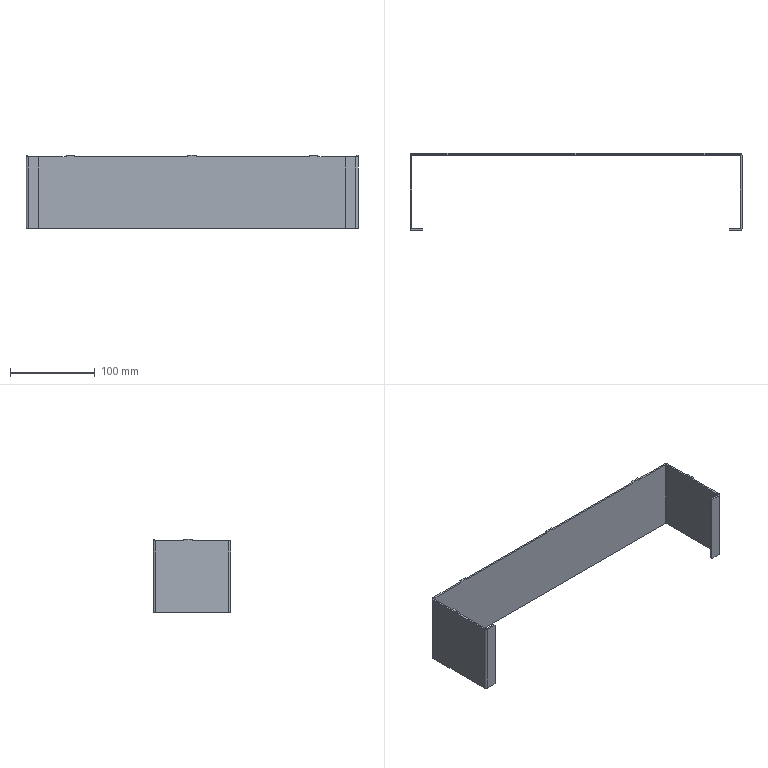Part | STEP file | xzz-002 | 1 solid | 42 faces | box 392 x 91.5 x 87 mm | volume 101252 mm3 | plane 34 | cylinder 8 | commonest cylinder face diameters 1 x4 5 x4
STEP:
#1=CARTESIAN_POINT('',(216.5,24.,85.));
#2=VERTEX_POINT('',#1);
#3=CARTESIAN_POINT('',(216.5,24.,0.));
#4=VERTEX_POINT('',#3);
#5=CARTESIAN_POINT('',(216.5,24.,85.));
#6=DIRECTION('',(0.,0.,-1.));
#7=VECTOR('',#6,1000.);
#8=LINE('',#5,#7);
#9=EDGE_CURVE('',#2,#4,#8,.T.);
#10=ORIENTED_EDGE('',*,*,#9,.F.);
#11=CARTESIAN_POINT('',(171.7,24.,85.));
#12=VERTEX_POINT('',#11);
#13=CARTESIAN_POINT('',(-173.,24.,85.));
#14=DIRECTION('',(1.,0.,0.));
#15=VECTOR('',#14,1000.);
#16=LINE('',#13,#15);
#17=EDGE_CURVE('',#12,#2,#16,.T.);
#18=ORIENTED_EDGE('',*,*,#17,.F.);
#19=CARTESIAN_POINT('',(171.7,24.,87.));
#20=VERTEX_POINT('',#19);
#21=CARTESIAN_POINT('',(171.7,24.,85.));
#22=DIRECTION('',(0.,0.,-1.));
#23=VECTOR('',#22,1000.);
#24=LINE('',#21,#23);
#25=EDGE_CURVE('',#20,#12,#24,.T.);
#26=ORIENTED_EDGE('',*,*,#25,.F.);
#27=CARTESIAN_POINT('',(161.7,24.,87.));
#28=VERTEX_POINT('',#27);
#29=CARTESIAN_POINT('',(-173.,24.,87.));
#30=DIRECTION('',(1.,0.,0.));
#31=VECTOR('',#30,1000.);
#32=LINE('',#29,#31);
#33=EDGE_CURVE('',#28,#20,#32,.T.);
#34=ORIENTED_EDGE('',*,*,#33,.F.);
#35=CARTESIAN_POINT('',(161.7,24.,85.));
#36=VERTEX_POINT('',#35);
#37=CARTESIAN_POINT('',(161.7,24.,85.));
#38=DIRECTION('',(0.,0.,1.));
#39=VECTOR('',#38,1000.);
#40=LINE('',#37,#39);
#41=EDGE_CURVE('',#36,#28,#40,.T.);
#42=ORIENTED_EDGE('',*,*,#41,.F.);
#43=CARTESIAN_POINT('',(28.,24.,85.));
#44=VERTEX_POINT('',#43);
#45=CARTESIAN_POINT('',(-173.,24.,85.));
#46=DIRECTION('',(1.,0.,0.));
#47=VECTOR('',#46,1000.);
#48=LINE('',#45,#47);
#49=EDGE_CURVE('',#44,#36,#48,.T.);
#50=ORIENTED_EDGE('',*,*,#49,.F.);
#51=CARTESIAN_POINT('',(28.,24.,87.));
#52=VERTEX_POINT('',#51);
#53=CARTESIAN_POINT('',(28.,24.,85.));
#54=DIRECTION('',(0.,0.,-1.));
#55=VECTOR('',#54,1000.);
#56=LINE('',#53,#55);
#57=EDGE_CURVE('',#52,#44,#56,.T.);
#58=ORIENTED_EDGE('',*,*,#57,.F.);
#59=CARTESIAN_POINT('',(18.,24.,87.));
#60=VERTEX_POINT('',#59);
#61=CARTESIAN_POINT('',(-173.,24.,87.));
#62=DIRECTION('',(1.,0.,0.));
#63=VECTOR('',#62,1000.);
#64=LINE('',#61,#63);
#65=EDGE_CURVE('',#60,#52,#64,.T.);
#66=ORIENTED_EDGE('',*,*,#65,.F.);
#67=CARTESIAN_POINT('',(18.,24.,85.));
#68=VERTEX_POINT('',#67);
#69=CARTESIAN_POINT('',(18.,24.,85.));
#70=DIRECTION('',(0.,0.,1.));
#71=VECTOR('',#70,1000.);
#72=LINE('',#69,#71);
#73=EDGE_CURVE('',#68,#60,#72,.T.);
#74=ORIENTED_EDGE('',*,*,#73,.F.);
#75=CARTESIAN_POINT('',(-115.7,24.,85.));
#76=VERTEX_POINT('',#75);
#77=CARTESIAN_POINT('',(-173.,24.,85.));
#78=DIRECTION('',(1.,0.,0.));
#79=VECTOR('',#78,1000.);
#80=LINE('',#77,#79);
#81=EDGE_CURVE('',#76,#68,#80,.T.);
#82=ORIENTED_EDGE('',*,*,#81,.F.);
#83=CARTESIAN_POINT('',(-115.7,24.,87.));
#84=VERTEX_POINT('',#83);
#85=CARTESIAN_POINT('',(-115.7,24.,85.));
#86=DIRECTION('',(0.,0.,-1.));
#87=VECTOR('',#86,1000.);
#88=LINE('',#85,#87);
#89=EDGE_CURVE('',#84,#76,#88,.T.);
#90=ORIENTED_EDGE('',*,*,#89,.F.);
#91=CARTESIAN_POINT('',(-125.7,24.,87.));
#92=VERTEX_POINT('',#91);
#93=CARTESIAN_POINT('',(-173.,24.,87.));
#94=DIRECTION('',(1.,0.,0.));
#95=VECTOR('',#94,1000.);
#96=LINE('',#93,#95);
#97=EDGE_CURVE('',#92,#84,#96,.T.);
#98=ORIENTED_EDGE('',*,*,#97,.F.);
#99=CARTESIAN_POINT('',(-125.7,24.,85.));
#100=VERTEX_POINT('',#99);
#101=CARTESIAN_POINT('',(-125.7,24.,85.));
#102=DIRECTION('',(0.,0.,1.));
#103=VECTOR('',#102,1000.);
#104=LINE('',#101,#103);
#105=EDGE_CURVE('',#100,#92,#104,.T.);
#106=ORIENTED_EDGE('',*,*,#105,.F.);
#107=CARTESIAN_POINT('',(-170.5,24.,85.));
#108=VERTEX_POINT('',#107);
#109=CARTESIAN_POINT('',(-173.,24.,85.));
#110=DIRECTION('',(1.,0.,0.));
#111=VECTOR('',#110,1000.);
#112=LINE('',#109,#111);
#113=EDGE_CURVE('',#108,#100,#112,.T.);
#114=ORIENTED_EDGE('',*,*,#113,.F.);
#115=CARTESIAN_POINT('',(-170.5,24.,0.));
#116=VERTEX_POINT('',#115);
#117=CARTESIAN_POINT('',(-170.5,24.,85.));
#118=DIRECTION('',(0.,0.,1.));
#119=VECTOR('',#118,1000.);
#120=LINE('',#117,#119);
#121=EDGE_CURVE('',#116,#108,#120,.T.);
#122=ORIENTED_EDGE('',*,*,#121,.F.);
#123=CARTESIAN_POINT('',(-173.,24.,0.));
#124=DIRECTION('',(-1.,0.,0.));
#125=VECTOR('',#124,1000.);
#126=LINE('',#123,#125);
#127=EDGE_CURVE('',#4,#116,#126,.T.);
#128=ORIENTED_EDGE('',*,*,#127,.F.);
#129=EDGE_LOOP('',(#10,#18,#26,#34,#42,#50,#58,#66,#74,#82,#90,#98,#106,#114,#122,#128));
#130=FACE_OUTER_BOUND('',#129,.T.);
#131=CARTESIAN_POINT('',(-173.,24.,85.));
#132=DIRECTION('',(0.,1.,0.));
#133=DIRECTION('',(0.,0.,1.));
#134=AXIS2_PLACEMENT_3D('',#131,#132,#133);
#135=PLANE('',#134);
#136=ADVANCED_FACE('',(#130),#135,.F.);
#137=ORIENTED_EDGE('',*,*,#127,.T.);
#138=CARTESIAN_POINT('',(-171.,23.5,0.));
#139=VERTEX_POINT('',#138);
#140=CARTESIAN_POINT('',(-170.5,23.5,0.));
#141=DIRECTION('',(0.,0.,1.));
#142=DIRECTION('',(-1.,0.,0.));
#143=AXIS2_PLACEMENT_3D('',#140,#141,#142);
#144=CIRCLE('',#143,0.5);
#145=EDGE_CURVE('',#116,#139,#144,.T.);
#146=ORIENTED_EDGE('',*,*,#145,.T.);
#147=CARTESIAN_POINT('',(-171.,-63.,0.));
#148=VERTEX_POINT('',#147);
#149=CARTESIAN_POINT('',(-171.,26.,0.));
#150=DIRECTION('',(0.,-1.,0.));
#151=VECTOR('',#150,1000.);
#152=LINE('',#149,#151);
#153=EDGE_CURVE('',#139,#148,#152,.T.);
#154=ORIENTED_EDGE('',*,*,#153,.T.);
#155=CARTESIAN_POINT('',(-170.5,-63.5,0.));
#156=VERTEX_POINT('',#155);
#157=CARTESIAN_POINT('',(-170.5,-63.,0.));
#158=DIRECTION('',(0.,0.,1.));
#159=DIRECTION('',(-1.,0.,0.));
#160=AXIS2_PLACEMENT_3D('',#157,#158,#159);
#161=CIRCLE('',#160,0.5);
#162=EDGE_CURVE('',#148,#156,#161,.T.);
#163=ORIENTED_EDGE('',*,*,#162,.T.);
#164=CARTESIAN_POINT('',(-158.,-63.5,0.));
#165=VERTEX_POINT('',#164);
#166=CARTESIAN_POINT('',(-173.,-63.5,0.));
#167=DIRECTION('',(1.,0.,0.));
#168=VECTOR('',#167,1000.);
#169=LINE('',#166,#168);
#170=EDGE_CURVE('',#156,#165,#169,.T.);
#171=ORIENTED_EDGE('',*,*,#170,.T.);
#172=CARTESIAN_POINT('',(-158.,-65.5,0.));
#173=VERTEX_POINT('',#172);
#174=CARTESIAN_POINT('',(-158.,-63.,0.));
#175=DIRECTION('',(0.,-1.,0.));
#176=VECTOR('',#175,1000.);
#177=LINE('',#174,#176);
#178=EDGE_CURVE('',#165,#173,#177,.T.);
#179=ORIENTED_EDGE('',*,*,#178,.T.);
#180=CARTESIAN_POINT('',(-170.5,-65.5,0.));
#181=VERTEX_POINT('',#180);
#182=CARTESIAN_POINT('',(-171.,-65.5,0.));
#183=DIRECTION('',(-1.,0.,0.));
#184=VECTOR('',#183,1000.);
#185=LINE('',#182,#184);
#186=EDGE_CURVE('',#173,#181,#185,.T.);
#187=ORIENTED_EDGE('',*,*,#186,.T.);
#188=CARTESIAN_POINT('',(-173.,-63.,0.));
#189=VERTEX_POINT('',#188);
#190=CARTESIAN_POINT('',(-170.5,-63.,0.));
#191=DIRECTION('',(0.,0.,-1.));
#192=DIRECTION('',(-1.,0.,0.));
#193=AXIS2_PLACEMENT_3D('',#190,#191,#192);
#194=CIRCLE('',#193,2.5);
#195=EDGE_CURVE('',#181,#189,#194,.T.);
#196=ORIENTED_EDGE('',*,*,#195,.T.);
#197=CARTESIAN_POINT('',(-173.,23.5,0.));
#198=VERTEX_POINT('',#197);
#199=CARTESIAN_POINT('',(-173.,24.,0.));
#200=DIRECTION('',(0.,1.,0.));
#201=VECTOR('',#200,1000.);
#202=LINE('',#199,#201);
#203=EDGE_CURVE('',#189,#198,#202,.T.);
#204=ORIENTED_EDGE('',*,*,#203,.T.);
#205=CARTESIAN_POINT('',(-170.5,26.,0.));
#206=VERTEX_POINT('',#205);
#207=CARTESIAN_POINT('',(-170.5,23.5,0.));
#208=DIRECTION('',(0.,0.,-1.));
#209=DIRECTION('',(-1.,0.,0.));
#210=AXIS2_PLACEMENT_3D('',#207,#208,#209);
#211=CIRCLE('',#210,2.5);
#212=EDGE_CURVE('',#198,#206,#211,.T.);
#213=ORIENTED_EDGE('',*,*,#212,.T.);
#214=CARTESIAN_POINT('',(216.5,26.,0.));
#215=VERTEX_POINT('',#214);
#216=CARTESIAN_POINT('',(217.,26.,0.));
#217=DIRECTION('',(1.,0.,0.));
#218=VECTOR('',#217,1000.);
#219=LINE('',#216,#218);
#220=EDGE_CURVE('',#206,#215,#219,.T.);
#221=ORIENTED_EDGE('',*,*,#220,.T.);
#222=CARTESIAN_POINT('',(219.,23.5,0.));
#223=VERTEX_POINT('',#222);
#224=CARTESIAN_POINT('',(216.5,23.5,0.));
#225=DIRECTION('',(0.,0.,-1.));
#226=DIRECTION('',(-1.,0.,0.));
#227=AXIS2_PLACEMENT_3D('',#224,#225,#226);
#228=CIRCLE('',#227,2.5);
#229=EDGE_CURVE('',#215,#223,#228,.T.);
#230=ORIENTED_EDGE('',*,*,#229,.T.);
#231=CARTESIAN_POINT('',(219.,-63.,0.));
#232=VERTEX_POINT('',#231);
#233=CARTESIAN_POINT('',(219.,-63.5,0.));
#234=DIRECTION('',(0.,-1.,0.));
#235=VECTOR('',#234,1000.);
#236=LINE('',#233,#235);
#237=EDGE_CURVE('',#223,#232,#236,.T.);
#238=ORIENTED_EDGE('',*,*,#237,.T.);
#239=CARTESIAN_POINT('',(216.5,-65.5,0.));
#240=VERTEX_POINT('',#239);
#241=CARTESIAN_POINT('',(216.5,-63.,0.));
#242=DIRECTION('',(0.,0.,-1.));
#243=DIRECTION('',(-1.,0.,0.));
#244=AXIS2_PLACEMENT_3D('',#241,#242,#243);
#245=CIRCLE('',#244,2.5);
#246=EDGE_CURVE('',#232,#240,#245,.T.);
#247=ORIENTED_EDGE('',*,*,#246,.T.);
#248=CARTESIAN_POINT('',(204.,-65.5,0.));
#249=VERTEX_POINT('',#248);
#250=CARTESIAN_POINT('',(216.5,-65.5,0.));
#251=DIRECTION('',(1.,0.,0.));
#252=VECTOR('',#251,1000.);
#253=LINE('',#250,#252);
#254=EDGE_CURVE('',#249,#240,#253,.T.);
#255=ORIENTED_EDGE('',*,*,#254,.F.);
#256=CARTESIAN_POINT('',(204.,-63.5,0.));
#257=VERTEX_POINT('',#256);
#258=CARTESIAN_POINT('',(204.,-63.,0.));
#259=DIRECTION('',(0.,-1.,0.));
#260=VECTOR('',#259,1000.);
#261=LINE('',#258,#260);
#262=EDGE_CURVE('',#257,#249,#261,.T.);
#263=ORIENTED_EDGE('',*,*,#262,.F.);
#264=CARTESIAN_POINT('',(216.5,-63.5,0.));
#265=VERTEX_POINT('',#264);
#266=CARTESIAN_POINT('',(219.,-63.5,0.));
#267=DIRECTION('',(1.,0.,0.));
#268=VECTOR('',#267,1000.);
#269=LINE('',#266,#268);
#270=EDGE_CURVE('',#257,#265,#269,.T.);
#271=ORIENTED_EDGE('',*,*,#270,.T.);
#272=CARTESIAN_POINT('',(217.,-63.,0.));
#273=VERTEX_POINT('',#272);
#274=CARTESIAN_POINT('',(216.5,-63.,0.));
#275=DIRECTION('',(0.,0.,1.));
#276=DIRECTION('',(-1.,0.,0.));
#277=AXIS2_PLACEMENT_3D('',#274,#275,#276);
#278=CIRCLE('',#277,0.5);
#279=EDGE_CURVE('',#265,#273,#278,.T.);
#280=ORIENTED_EDGE('',*,*,#279,.T.);
#281=CARTESIAN_POINT('',(217.,23.5,0.));
#282=VERTEX_POINT('',#281);
#283=CARTESIAN_POINT('',(217.,26.,0.));
#284=DIRECTION('',(0.,1.,0.));
#285=VECTOR('',#284,1000.);
#286=LINE('',#283,#285);
#287=EDGE_CURVE('',#273,#282,#286,.T.);
#288=ORIENTED_EDGE('',*,*,#287,.T.);
#289=CARTESIAN_POINT('',(216.5,23.5,0.));
#290=DIRECTION('',(0.,0.,1.));
#291=DIRECTION('',(-1.,0.,0.));
#292=AXIS2_PLACEMENT_3D('',#289,#290,#291);
#293=CIRCLE('',#292,0.5);
#294=EDGE_CURVE('',#282,#4,#293,.T.);
#295=ORIENTED_EDGE('',*,*,#294,.T.);
#296=EDGE_LOOP('',(#137,#146,#154,#163,#171,#179,#187,#196,#204,#213,#221,#230,#238,#247,#255,#263,#271,#280,#288,#295));
#297=FACE_OUTER_BOUND('',#296,.T.);
#298=CARTESIAN_POINT('',(217.,23.5,0.));
#299=DIRECTION('',(0.,0.,-1.));
#300=DIRECTION('',(-1.,0.,0.));
#301=AXIS2_PLACEMENT_3D('',#298,#299,#300);
#302=PLANE('',#301);
#303=ADVANCED_FACE('',(#297),#302,.T.);
#304=CARTESIAN_POINT('',(217.,23.5,85.));
#305=VERTEX_POINT('',#304);
#306=CARTESIAN_POINT('',(217.,23.5,85.));
#307=DIRECTION('',(0.,0.,-1.));
#308=VECTOR('',#307,1000.);
#309=LINE('',#306,#308);
#310=EDGE_CURVE('',#305,#282,#309,.T.);
#311=ORIENTED_EDGE('',*,*,#310,.F.);
#312=CARTESIAN_POINT('',(216.5,23.5,85.));
#313=DIRECTION('',(0.,0.,-1.));
#314=DIRECTION('',(-1.,0.,0.));
#315=AXIS2_PLACEMENT_3D('',#312,#313,#314);
#316=CIRCLE('',#315,0.5);
#317=EDGE_CURVE('',#2,#305,#316,.T.);
#318=ORIENTED_EDGE('',*,*,#317,.F.);
#319=ORIENTED_EDGE('',*,*,#9,.T.);
#320=ORIENTED_EDGE('',*,*,#294,.F.);
#321=EDGE_LOOP('',(#311,#318,#319,#320));
#322=FACE_OUTER_BOUND('',#321,.T.);
#323=CARTESIAN_POINT('',(216.5,23.5,85.));
#324=DIRECTION('',(0.,0.,-1.));
#325=DIRECTION('',(-1.,0.,0.));
#326=AXIS2_PLACEMENT_3D('',#323,#324,#325);
#327=CYLINDRICAL_SURFACE('',#326,0.5);
#328=ADVANCED_FACE('',(#322),#327,.F.);
#329=ORIENTED_EDGE('',*,*,#17,.T.);
#330=ORIENTED_EDGE('',*,*,#317,.T.);
#331=CARTESIAN_POINT('',(217.,-10.,85.));
#332=VERTEX_POINT('',#331);
#333=CARTESIAN_POINT('',(217.,26.,85.));
#334=DIRECTION('',(0.,-1.,0.));
#335=VECTOR('',#334,1000.);
#336=LINE('',#333,#335);
#337=EDGE_CURVE('',#305,#332,#336,.T.);
#338=ORIENTED_EDGE('',*,*,#337,.T.);
#339=CARTESIAN_POINT('',(219.,-10.,85.));
#340=VERTEX_POINT('',#339);
#341=CARTESIAN_POINT('',(217.,-10.,85.));
#342=DIRECTION('',(1.,0.,0.));
#343=VECTOR('',#342,1000.);
#344=LINE('',#341,#343);
#345=EDGE_CURVE('',#332,#340,#344,.T.);
#346=ORIENTED_EDGE('',*,*,#345,.T.);
#347=CARTESIAN_POINT('',(219.,23.5,85.));
#348=VERTEX_POINT('',#347);
#349=CARTESIAN_POINT('',(219.,24.,85.));
#350=DIRECTION('',(0.,1.,0.));
#351=VECTOR('',#350,1000.);
#352=LINE('',#349,#351);
#353=EDGE_CURVE('',#340,#348,#352,.T.);
#354=ORIENTED_EDGE('',*,*,#353,.T.);
#355=CARTESIAN_POINT('',(216.5,26.,85.));
#356=VERTEX_POINT('',#355);
#357=CARTESIAN_POINT('',(216.5,23.5,85.));
#358=DIRECTION('',(0.,0.,1.));
#359=DIRECTION('',(-1.,0.,0.));
#360=AXIS2_PLACEMENT_3D('',#357,#358,#359);
#361=CIRCLE('',#360,2.5);
#362=EDGE_CURVE('',#348,#356,#361,.T.);
#363=ORIENTED_EDGE('',*,*,#362,.T.);
#364=CARTESIAN_POINT('',(171.7,26.,85.));
#365=VERTEX_POINT('',#364);
#366=CARTESIAN_POINT('',(-171.,26.,85.));
#367=DIRECTION('',(-1.,0.,0.));
#368=VECTOR('',#367,1000.);
#369=LINE('',#366,#368);
#370=EDGE_CURVE('',#356,#365,#369,.T.);
#371=ORIENTED_EDGE('',*,*,#370,.T.);
#372=CARTESIAN_POINT('',(171.7,23.5,85.));
#373=DIRECTION('',(0.,-1.,0.));
#374=VECTOR('',#373,1000.);
#375=LINE('',#372,#374);
#376=EDGE_CURVE('',#365,#12,#375,.T.);
#377=ORIENTED_EDGE('',*,*,#376,.T.);
#378=EDGE_LOOP('',(#329,#330,#338,#346,#354,#363,#371,#377));
#379=FACE_OUTER_BOUND('',#378,.T.);
#380=CARTESIAN_POINT('',(-171.,23.5,85.));
#381=DIRECTION('',(0.,0.,1.));
#382=DIRECTION('',(1.,0.,0.));
#383=AXIS2_PLACEMENT_3D('',#380,#381,#382);
#384=PLANE('',#383);
#385=ADVANCED_FACE('',(#379),#384,.T.);
#386=CARTESIAN_POINT('',(171.7,26.,87.));
#387=VERTEX_POINT('',#386);
#388=CARTESIAN_POINT('',(171.7,26.,87.));
#389=DIRECTION('',(0.,0.,-1.));
#390=VECTOR('',#389,1000.);
#391=LINE('',#388,#390);
#392=EDGE_CURVE('',#387,#365,#391,.T.);
#393=ORIENTED_EDGE('',*,*,#392,.F.);
#394=CARTESIAN_POINT('',(171.7,26.,87.));
#395=DIRECTION('',(0.,1.,0.));
#396=VECTOR('',#395,1000.);
#397=LINE('',#394,#396);
#398=EDGE_CURVE('',#20,#387,#397,.T.);
#399=ORIENTED_EDGE('',*,*,#398,.F.);
#400=ORIENTED_EDGE('',*,*,#25,.T.);
#401=ORIENTED_EDGE('',*,*,#376,.F.);
#402=EDGE_LOOP('',(#393,#399,#400,#401));
#403=FACE_OUTER_BOUND('',#402,.T.);
#404=CARTESIAN_POINT('',(171.7,26.,87.));
#405=DIRECTION('',(-1.,0.,0.));
#406=DIRECTION('',(0.,0.,1.));
#407=AXIS2_PLACEMENT_3D('',#404,#405,#406);
#408=PLANE('',#407);
#409=ADVANCED_FACE('',(#403),#408,.F.);
#410=ORIENTED_EDGE('',*,*,#398,.T.);
#411=CARTESIAN_POINT('',(161.7,26.,87.));
#412=VERTEX_POINT('',#411);
#413=CARTESIAN_POINT('',(0.,26.,87.));
#414=DIRECTION('',(-1.,0.,0.));
#415=VECTOR('',#414,1000.);
#416=LINE('',#413,#415);
#417=EDGE_CURVE('',#387,#412,#416,.T.);
#418=ORIENTED_EDGE('',*,*,#417,.T.);
#419=CARTESIAN_POINT('',(161.7,0.,87.));
#420=DIRECTION('',(0.,-1.,0.));
#421=VECTOR('',#420,1000.);
#422=LINE('',#419,#421);
#423=EDGE_CURVE('',#412,#28,#422,.T.);
#424=ORIENTED_EDGE('',*,*,#423,.T.);
#425=ORIENTED_EDGE('',*,*,#33,.T.);
#426=EDGE_LOOP('',(#410,#418,#424,#425));
#427=FACE_OUTER_BOUND('',#426,.T.);
#428=CARTESIAN_POINT('',(0.,0.,87.));
#429=DIRECTION('',(0.,0.,1.));
#430=DIRECTION('',(1.,0.,0.));
#431=AXIS2_PLACEMENT_3D('',#428,#429,#430);
#432=PLANE('',#431);
#433=ADVANCED_FACE('',(#427),#432,.T.);
#434=ORIENTED_EDGE('',*,*,#41,.T.);
#435=ORIENTED_EDGE('',*,*,#423,.F.);
#436=CARTESIAN_POINT('',(161.7,26.,85.));
#437=VERTEX_POINT('',#436);
#438=CARTESIAN_POINT('',(161.7,26.,87.));
#439=DIRECTION('',(0.,0.,1.));
#440=VECTOR('',#439,1000.);
#441=LINE('',#438,#440);
#442=EDGE_CURVE('',#437,#412,#441,.T.);
#443=ORIENTED_EDGE('',*,*,#442,.F.);
#444=CARTESIAN_POINT('',(161.7,26.,85.));
#445=DIRECTION('',(0.,1.,0.));
#446=VECTOR('',#445,1000.);
#447=LINE('',#444,#446);
#448=EDGE_CURVE('',#36,#437,#447,.T.);
#449=ORIENTED_EDGE('',*,*,#448,.F.);
#450=EDGE_LOOP('',(#434,#435,#443,#449));
#451=FACE_OUTER_BOUND('',#450,.T.);
#452=CARTESIAN_POINT('',(161.7,26.,87.));
#453=DIRECTION('',(1.,0.,0.));
#454=DIRECTION('',(0.,0.,-1.));
#455=AXIS2_PLACEMENT_3D('',#452,#453,#454);
#456=PLANE('',#455);
#457=ADVANCED_FACE('',(#451),#456,.F.);
#458=CARTESIAN_POINT('',(28.,26.,85.));
#459=VERTEX_POINT('',#458);
#460=CARTESIAN_POINT('',(-171.,26.,85.));
#461=DIRECTION('',(-1.,0.,0.));
#462=VECTOR('',#461,1000.);
#463=LINE('',#460,#462);
#464=EDGE_CURVE('',#437,#459,#463,.T.);
#465=ORIENTED_EDGE('',*,*,#464,.T.);
#466=CARTESIAN_POINT('',(28.,23.5,85.));
#467=DIRECTION('',(0.,-1.,0.));
#468=VECTOR('',#467,1000.);
#469=LINE('',#466,#468);
#470=EDGE_CURVE('',#459,#44,#469,.T.);
#471=ORIENTED_EDGE('',*,*,#470,.T.);
#472=ORIENTED_EDGE('',*,*,#49,.T.);
#473=ORIENTED_EDGE('',*,*,#448,.T.);
#474=EDGE_LOOP('',(#465,#471,#472,#473));
#475=FACE_OUTER_BOUND('',#474,.T.);
#476=CARTESIAN_POINT('',(-171.,23.5,85.));
#477=DIRECTION('',(0.,0.,1.));
#478=DIRECTION('',(1.,0.,0.));
#479=AXIS2_PLACEMENT_3D('',#476,#477,#478);
#480=PLANE('',#479);
#481=ADVANCED_FACE('',(#475),#480,.T.);
#482=CARTESIAN_POINT('',(28.,26.,87.));
#483=VERTEX_POINT('',#482);
#484=CARTESIAN_POINT('',(28.,26.,87.));
#485=DIRECTION('',(0.,0.,-1.));
#486=VECTOR('',#485,1000.);
#487=LINE('',#484,#486);
#488=EDGE_CURVE('',#483,#459,#487,.T.);
#489=ORIENTED_EDGE('',*,*,#488,.F.);
#490=CARTESIAN_POINT('',(28.,26.,87.));
#491=DIRECTION('',(0.,1.,0.));
#492=VECTOR('',#491,1000.);
#493=LINE('',#490,#492);
#494=EDGE_CURVE('',#52,#483,#493,.T.);
#495=ORIENTED_EDGE('',*,*,#494,.F.);
#496=ORIENTED_EDGE('',*,*,#57,.T.);
#497=ORIENTED_EDGE('',*,*,#470,.F.);
#498=EDGE_LOOP('',(#489,#495,#496,#497));
#499=FACE_OUTER_BOUND('',#498,.T.);
#500=CARTESIAN_POINT('',(28.,26.,87.));
#501=DIRECTION('',(-1.,0.,0.));
#502=DIRECTION('',(0.,0.,1.));
#503=AXIS2_PLACEMENT_3D('',#500,#501,#502);
#504=PLANE('',#503);
#505=ADVANCED_FACE('',(#499),#504,.F.);
#506=ORIENTED_EDGE('',*,*,#494,.T.);
#507=CARTESIAN_POINT('',(18.,26.,87.));
#508=VERTEX_POINT('',#507);
#509=CARTESIAN_POINT('',(0.,26.,87.));
#510=DIRECTION('',(-1.,0.,0.));
#511=VECTOR('',#510,1000.);
#512=LINE('',#509,#511);
#513=EDGE_CURVE('',#483,#508,#512,.T.);
#514=ORIENTED_EDGE('',*,*,#513,.T.);
#515=CARTESIAN_POINT('',(18.,0.,87.));
#516=DIRECTION('',(0.,-1.,0.));
#517=VECTOR('',#516,1000.);
#518=LINE('',#515,#517);
#519=EDGE_CURVE('',#508,#60,#518,.T.);
#520=ORIENTED_EDGE('',*,*,#519,.T.);
#521=ORIENTED_EDGE('',*,*,#65,.T.);
#522=EDGE_LOOP('',(#506,#514,#520,#521));
#523=FACE_OUTER_BOUND('',#522,.T.);
#524=CARTESIAN_POINT('',(0.,0.,87.));
#525=DIRECTION('',(0.,0.,1.));
#526=DIRECTION('',(1.,0.,0.));
#527=AXIS2_PLACEMENT_3D('',#524,#525,#526);
#528=PLANE('',#527);
#529=ADVANCED_FACE('',(#523),#528,.T.);
#530=ORIENTED_EDGE('',*,*,#73,.T.);
#531=ORIENTED_EDGE('',*,*,#519,.F.);
#532=CARTESIAN_POINT('',(18.,26.,85.));
#533=VERTEX_POINT('',#532);
#534=CARTESIAN_POINT('',(18.,26.,87.));
#535=DIRECTION('',(0.,0.,1.));
#536=VECTOR('',#535,1000.);
#537=LINE('',#534,#536);
#538=EDGE_CURVE('',#533,#508,#537,.T.);
#539=ORIENTED_EDGE('',*,*,#538,.F.);
#540=CARTESIAN_POINT('',(18.,26.,85.));
#541=DIRECTION('',(0.,1.,0.));
#542=VECTOR('',#541,1000.);
#543=LINE('',#540,#542);
#544=EDGE_CURVE('',#68,#533,#543,.T.);
#545=ORIENTED_EDGE('',*,*,#544,.F.);
#546=EDGE_LOOP('',(#530,#531,#539,#545));
#547=FACE_OUTER_BOUND('',#546,.T.);
#548=CARTESIAN_POINT('',(18.,26.,87.));
#549=DIRECTION('',(1.,0.,0.));
#550=DIRECTION('',(0.,0.,-1.));
#551=AXIS2_PLACEMENT_3D('',#548,#549,#550);
#552=PLANE('',#551);
#553=ADVANCED_FACE('',(#547),#552,.F.);
#554=CARTESIAN_POINT('',(-115.7,26.,85.));
#555=VERTEX_POINT('',#554);
#556=CARTESIAN_POINT('',(-171.,26.,85.));
#557=DIRECTION('',(-1.,0.,0.));
#558=VECTOR('',#557,1000.);
#559=LINE('',#556,#558);
#560=EDGE_CURVE('',#533,#555,#559,.T.);
#561=ORIENTED_EDGE('',*,*,#560,.T.);
#562=CARTESIAN_POINT('',(-115.7,23.5,85.));
#563=DIRECTION('',(0.,-1.,0.));
#564=VECTOR('',#563,1000.);
#565=LINE('',#562,#564);
#566=EDGE_CURVE('',#555,#76,#565,.T.);
#567=ORIENTED_EDGE('',*,*,#566,.T.);
#568=ORIENTED_EDGE('',*,*,#81,.T.);
#569=ORIENTED_EDGE('',*,*,#544,.T.);
#570=EDGE_LOOP('',(#561,#567,#568,#569));
#571=FACE_OUTER_BOUND('',#570,.T.);
#572=CARTESIAN_POINT('',(-171.,23.5,85.));
#573=DIRECTION('',(0.,0.,1.));
#574=DIRECTION('',(1.,0.,0.));
#575=AXIS2_PLACEMENT_3D('',#572,#573,#574);
#576=PLANE('',#575);
#577=ADVANCED_FACE('',(#571),#576,.T.);
#578=CARTESIAN_POINT('',(-115.7,26.,87.));
#579=VERTEX_POINT('',#578);
#580=CARTESIAN_POINT('',(-115.7,26.,87.));
#581=DIRECTION('',(0.,0.,-1.));
#582=VECTOR('',#581,1000.);
#583=LINE('',#580,#582);
#584=EDGE_CURVE('',#579,#555,#583,.T.);
#585=ORIENTED_EDGE('',*,*,#584,.F.);
#586=CARTESIAN_POINT('',(-115.7,26.,87.));
#587=DIRECTION('',(0.,1.,0.));
#588=VECTOR('',#587,1000.);
#589=LINE('',#586,#588);
#590=EDGE_CURVE('',#84,#579,#589,.T.);
#591=ORIENTED_EDGE('',*,*,#590,.F.);
#592=ORIENTED_EDGE('',*,*,#89,.T.);
#593=ORIENTED_EDGE('',*,*,#566,.F.);
#594=EDGE_LOOP('',(#585,#591,#592,#593));
#595=FACE_OUTER_BOUND('',#594,.T.);
#596=CARTESIAN_POINT('',(-115.7,26.,87.));
#597=DIRECTION('',(-1.,0.,0.));
#598=DIRECTION('',(0.,0.,1.));
#599=AXIS2_PLACEMENT_3D('',#596,#597,#598);
#600=PLANE('',#599);
#601=ADVANCED_FACE('',(#595),#600,.F.);
#602=ORIENTED_EDGE('',*,*,#590,.T.);
#603=CARTESIAN_POINT('',(-125.7,26.,87.));
#604=VERTEX_POINT('',#603);
#605=CARTESIAN_POINT('',(0.,26.,87.));
#606=DIRECTION('',(-1.,0.,0.));
#607=VECTOR('',#606,1000.);
#608=LINE('',#605,#607);
#609=EDGE_CURVE('',#579,#604,#608,.T.);
#610=ORIENTED_EDGE('',*,*,#609,.T.);
#611=CARTESIAN_POINT('',(-125.7,0.,87.));
#612=DIRECTION('',(0.,-1.,0.));
#613=VECTOR('',#612,1000.);
#614=LINE('',#611,#613);
#615=EDGE_CURVE('',#604,#92,#614,.T.);
#616=ORIENTED_EDGE('',*,*,#615,.T.);
#617=ORIENTED_EDGE('',*,*,#97,.T.);
#618=EDGE_LOOP('',(#602,#610,#616,#617));
#619=FACE_OUTER_BOUND('',#618,.T.);
#620=CARTESIAN_POINT('',(0.,0.,87.));
#621=DIRECTION('',(0.,0.,1.));
#622=DIRECTION('',(1.,0.,0.));
#623=AXIS2_PLACEMENT_3D('',#620,#621,#622);
#624=PLANE('',#623);
#625=ADVANCED_FACE('',(#619),#624,.T.);
#626=ORIENTED_EDGE('',*,*,#105,.T.);
#627=ORIENTED_EDGE('',*,*,#615,.F.);
#628=CARTESIAN_POINT('',(-125.7,26.,85.));
#629=VERTEX_POINT('',#628);
#630=CARTESIAN_POINT('',(-125.7,26.,87.));
#631=DIRECTION('',(0.,0.,1.));
#632=VECTOR('',#631,1000.);
#633=LINE('',#630,#632);
#634=EDGE_CURVE('',#629,#604,#633,.T.);
#635=ORIENTED_EDGE('',*,*,#634,.F.);
#636=CARTESIAN_POINT('',(-125.7,26.,85.));
#637=DIRECTION('',(0.,1.,0.));
#638=VECTOR('',#637,1000.);
#639=LINE('',#636,#638);
#640=EDGE_CURVE('',#100,#629,#639,.T.);
#641=ORIENTED_EDGE('',*,*,#640,.F.);
#642=EDGE_LOOP('',(#626,#627,#635,#641));
#643=FACE_OUTER_BOUND('',#642,.T.);
#644=CARTESIAN_POINT('',(-125.7,26.,87.));
#645=DIRECTION('',(1.,0.,0.));
#646=DIRECTION('',(0.,0.,-1.));
#647=AXIS2_PLACEMENT_3D('',#644,#645,#646);
#648=PLANE('',#647);
#649=ADVANCED_FACE('',(#643),#648,.F.);
#650=CARTESIAN_POINT('',(-170.5,26.,85.));
#651=VERTEX_POINT('',#650);
#652=CARTESIAN_POINT('',(-171.,26.,85.));
#653=DIRECTION('',(-1.,0.,0.));
#654=VECTOR('',#653,1000.);
#655=LINE('',#652,#654);
#656=EDGE_CURVE('',#629,#651,#655,.T.);
#657=ORIENTED_EDGE('',*,*,#656,.T.);
#658=CARTESIAN_POINT('',(-173.,23.5,85.));
#659=VERTEX_POINT('',#658);
#660=CARTESIAN_POINT('',(-170.5,23.5,85.));
#661=DIRECTION('',(0.,0.,1.));
#662=DIRECTION('',(-1.,0.,0.));
#663=AXIS2_PLACEMENT_3D('',#660,#661,#662);
#664=CIRCLE('',#663,2.5);
#665=EDGE_CURVE('',#651,#659,#664,.T.);
#666=ORIENTED_EDGE('',*,*,#665,.T.);
#667=CARTESIAN_POINT('',(-173.,-10.,85.));
#668=VERTEX_POINT('',#667);
#669=CARTESIAN_POINT('',(-173.,-63.5,85.));
#670=DIRECTION('',(0.,-1.,0.));
#671=VECTOR('',#670,1000.);
#672=LINE('',#669,#671);
#673=EDGE_CURVE('',#659,#668,#672,.T.);
#674=ORIENTED_EDGE('',*,*,#673,.T.);
#675=CARTESIAN_POINT('',(-171.,-10.,85.));
#676=VERTEX_POINT('',#675);
#677=CARTESIAN_POINT('',(-170.5,-10.,85.));
#678=DIRECTION('',(1.,0.,0.));
#679=VECTOR('',#678,1000.);
#680=LINE('',#677,#679);
#681=EDGE_CURVE('',#668,#676,#680,.T.);
#682=ORIENTED_EDGE('',*,*,#681,.T.);
#683=CARTESIAN_POINT('',(-171.,23.5,85.));
#684=VERTEX_POINT('',#683);
#685=CARTESIAN_POINT('',(-171.,26.,85.));
#686=DIRECTION('',(0.,1.,0.));
#687=VECTOR('',#686,1000.);
#688=LINE('',#685,#687);
#689=EDGE_CURVE('',#676,#684,#688,.T.);
#690=ORIENTED_EDGE('',*,*,#689,.T.);
#691=CARTESIAN_POINT('',(-170.5,23.5,85.));
#692=DIRECTION('',(0.,0.,-1.));
#693=DIRECTION('',(-1.,0.,0.));
#694=AXIS2_PLACEMENT_3D('',#691,#692,#693);
#695=CIRCLE('',#694,0.5);
#696=EDGE_CURVE('',#684,#108,#695,.T.);
#697=ORIENTED_EDGE('',*,*,#696,.T.);
#698=ORIENTED_EDGE('',*,*,#113,.T.);
#699=ORIENTED_EDGE('',*,*,#640,.T.);
#700=EDGE_LOOP('',(#657,#666,#674,#682,#690,#697,#698,#699));
#701=FACE_OUTER_BOUND('',#700,.T.);
#702=CARTESIAN_POINT('',(-171.,23.5,85.));
#703=DIRECTION('',(0.,0.,1.));
#704=DIRECTION('',(1.,0.,0.));
#705=AXIS2_PLACEMENT_3D('',#702,#703,#704);
#706=PLANE('',#705);
#707=ADVANCED_FACE('',(#701),#706,.T.);
#708=ORIENTED_EDGE('',*,*,#121,.T.);
#709=ORIENTED_EDGE('',*,*,#696,.F.);
#710=CARTESIAN_POINT('',(-171.,23.5,85.));
#711=DIRECTION('',(0.,0.,1.));
#712=VECTOR('',#711,1000.);
#713=LINE('',#710,#712);
#714=EDGE_CURVE('',#139,#684,#713,.T.);
#715=ORIENTED_EDGE('',*,*,#714,.F.);
#716=ORIENTED_EDGE('',*,*,#145,.F.);
#717=EDGE_LOOP('',(#708,#709,#715,#716));
#718=FACE_OUTER_BOUND('',#717,.T.);
#719=CARTESIAN_POINT('',(-170.5,23.5,85.));
#720=DIRECTION('',(0.,0.,-1.));
#721=DIRECTION('',(-1.,0.,0.));
#722=AXIS2_PLACEMENT_3D('',#719,#720,#721);
#723=CYLINDRICAL_SURFACE('',#722,0.5);
#724=ADVANCED_FACE('',(#718),#723,.F.);
#725=ORIENTED_EDGE('',*,*,#370,.F.);
#726=CARTESIAN_POINT('',(216.5,26.,85.));
#727=DIRECTION('',(0.,0.,-1.));
#728=VECTOR('',#727,1000.);
#729=LINE('',#726,#728);
#730=EDGE_CURVE('',#356,#215,#729,.T.);
#731=ORIENTED_EDGE('',*,*,#730,.T.);
#732=ORIENTED_EDGE('',*,*,#220,.F.);
#733=CARTESIAN_POINT('',(-170.5,26.,85.));
#734=DIRECTION('',(0.,0.,1.));
#735=VECTOR('',#734,1000.);
#736=LINE('',#733,#735);
#737=EDGE_CURVE('',#206,#651,#736,.T.);
#738=ORIENTED_EDGE('',*,*,#737,.T.);
#739=ORIENTED_EDGE('',*,*,#656,.F.);
#740=ORIENTED_EDGE('',*,*,#634,.T.);
#741=ORIENTED_EDGE('',*,*,#609,.F.);
#742=ORIENTED_EDGE('',*,*,#584,.T.);
#743=ORIENTED_EDGE('',*,*,#560,.F.);
#744=ORIENTED_EDGE('',*,*,#538,.T.);
#745=ORIENTED_EDGE('',*,*,#513,.F.);
#746=ORIENTED_EDGE('',*,*,#488,.T.);
#747=ORIENTED_EDGE('',*,*,#464,.F.);
#748=ORIENTED_EDGE('',*,*,#442,.T.);
#749=ORIENTED_EDGE('',*,*,#417,.F.);
#750=ORIENTED_EDGE('',*,*,#392,.T.);
#751=EDGE_LOOP('',(#725,#731,#732,#738,#739,#740,#741,#742,#743,#744,#745,#746,#747,#748,#749,#750));
#752=FACE_OUTER_BOUND('',#751,.T.);
#753=CARTESIAN_POINT('',(-173.,26.,85.));
#754=DIRECTION('',(0.,1.,0.));
#755=DIRECTION('',(0.,0.,1.));
#756=AXIS2_PLACEMENT_3D('',#753,#754,#755);
#757=PLANE('',#756);
#758=ADVANCED_FACE('',(#752),#757,.T.);
#759=CARTESIAN_POINT('',(217.,-63.,85.));
#760=VERTEX_POINT('',#759);
#761=CARTESIAN_POINT('',(217.,-63.,85.));
#762=DIRECTION('',(0.,0.,-1.));
#763=VECTOR('',#762,1000.);
#764=LINE('',#761,#763);
#765=EDGE_CURVE('',#760,#273,#764,.T.);
#766=ORIENTED_EDGE('',*,*,#765,.F.);
#767=CARTESIAN_POINT('',(217.,-20.,85.));
#768=VERTEX_POINT('',#767);
#769=CARTESIAN_POINT('',(217.,26.,85.));
#770=DIRECTION('',(0.,-1.,0.));
#771=VECTOR('',#770,1000.);
#772=LINE('',#769,#771);
#773=EDGE_CURVE('',#768,#760,#772,.T.);
#774=ORIENTED_EDGE('',*,*,#773,.F.);
#775=CARTESIAN_POINT('',(217.,-20.,87.));
#776=VERTEX_POINT('',#775);
#777=CARTESIAN_POINT('',(217.,-20.,85.));
#778=DIRECTION('',(0.,0.,-1.));
#779=VECTOR('',#778,1000.);
#780=LINE('',#777,#779);
#781=EDGE_CURVE('',#776,#768,#780,.T.);
#782=ORIENTED_EDGE('',*,*,#781,.F.);
#783=CARTESIAN_POINT('',(217.,-10.,87.));
#784=VERTEX_POINT('',#783);
#785=CARTESIAN_POINT('',(217.,26.,87.));
#786=DIRECTION('',(0.,-1.,0.));
#787=VECTOR('',#786,1000.);
#788=LINE('',#785,#787);
#789=EDGE_CURVE('',#784,#776,#788,.T.);
#790=ORIENTED_EDGE('',*,*,#789,.F.);
#791=CARTESIAN_POINT('',(217.,-10.,85.));
#792=DIRECTION('',(0.,0.,1.));
#793=VECTOR('',#792,1000.);
#794=LINE('',#791,#793);
#795=EDGE_CURVE('',#332,#784,#794,.T.);
#796=ORIENTED_EDGE('',*,*,#795,.F.);
#797=ORIENTED_EDGE('',*,*,#337,.F.);
#798=ORIENTED_EDGE('',*,*,#310,.T.);
#799=ORIENTED_EDGE('',*,*,#287,.F.);
#800=EDGE_LOOP('',(#766,#774,#782,#790,#796,#797,#798,#799));
#801=FACE_OUTER_BOUND('',#800,.T.);
#802=CARTESIAN_POINT('',(217.,26.,85.));
#803=DIRECTION('',(1.,0.,0.));
#804=DIRECTION('',(0.,0.,-1.));
#805=AXIS2_PLACEMENT_3D('',#802,#803,#804);
#806=PLANE('',#805);
#807=ADVANCED_FACE('',(#801),#806,.F.);
#808=ORIENTED_EDGE('',*,*,#714,.T.);
#809=ORIENTED_EDGE('',*,*,#689,.F.);
#810=CARTESIAN_POINT('',(-171.,-10.,87.));
#811=VERTEX_POINT('',#810);
#812=CARTESIAN_POINT('',(-171.,-10.,85.));
#813=DIRECTION('',(0.,0.,-1.));
#814=VECTOR('',#813,1000.);
#815=LINE('',#812,#814);
#816=EDGE_CURVE('',#811,#676,#815,.T.);
#817=ORIENTED_EDGE('',*,*,#816,.F.);
#818=CARTESIAN_POINT('',(-171.,-20.,87.));
#819=VERTEX_POINT('',#818);
#820=CARTESIAN_POINT('',(-171.,26.,87.));
#821=DIRECTION('',(0.,1.,0.));
#822=VECTOR('',#821,1000.);
#823=LINE('',#820,#822);
#824=EDGE_CURVE('',#819,#811,#823,.T.);
#825=ORIENTED_EDGE('',*,*,#824,.F.);
#826=CARTESIAN_POINT('',(-171.,-20.,85.));
#827=VERTEX_POINT('',#826);
#828=CARTESIAN_POINT('',(-171.,-20.,85.));
#829=DIRECTION('',(0.,0.,1.));
#830=VECTOR('',#829,1000.);
#831=LINE('',#828,#830);
#832=EDGE_CURVE('',#827,#819,#831,.T.);
#833=ORIENTED_EDGE('',*,*,#832,.F.);
#834=CARTESIAN_POINT('',(-171.,-63.,85.));
#835=VERTEX_POINT('',#834);
#836=CARTESIAN_POINT('',(-171.,26.,85.));
#837=DIRECTION('',(0.,1.,0.));
#838=VECTOR('',#837,1000.);
#839=LINE('',#836,#838);
#840=EDGE_CURVE('',#835,#827,#839,.T.);
#841=ORIENTED_EDGE('',*,*,#840,.F.);
#842=CARTESIAN_POINT('',(-171.,-63.,85.));
#843=DIRECTION('',(0.,0.,1.));
#844=VECTOR('',#843,1000.);
#845=LINE('',#842,#844);
#846=EDGE_CURVE('',#148,#835,#845,.T.);
#847=ORIENTED_EDGE('',*,*,#846,.F.);
#848=ORIENTED_EDGE('',*,*,#153,.F.);
#849=EDGE_LOOP('',(#808,#809,#817,#825,#833,#841,#847,#848));
#850=FACE_OUTER_BOUND('',#849,.T.);
#851=CARTESIAN_POINT('',(-171.,26.,85.));
#852=DIRECTION('',(-1.,0.,0.));
#853=DIRECTION('',(0.,0.,1.));
#854=AXIS2_PLACEMENT_3D('',#851,#852,#853);
#855=PLANE('',#854);
#856=ADVANCED_FACE('',(#850),#855,.F.);
#857=ORIENTED_EDGE('',*,*,#665,.F.);
#858=ORIENTED_EDGE('',*,*,#737,.F.);
#859=ORIENTED_EDGE('',*,*,#212,.F.);
#860=CARTESIAN_POINT('',(-173.,23.5,85.));
#861=DIRECTION('',(0.,0.,1.));
#862=VECTOR('',#861,1000.);
#863=LINE('',#860,#862);
#864=EDGE_CURVE('',#198,#659,#863,.T.);
#865=ORIENTED_EDGE('',*,*,#864,.T.);
#866=EDGE_LOOP('',(#857,#858,#859,#865));
#867=FACE_OUTER_BOUND('',#866,.T.);
#868=CARTESIAN_POINT('',(-170.5,23.5,85.));
#869=DIRECTION('',(0.,0.,-1.));
#870=DIRECTION('',(-1.,0.,0.));
#871=AXIS2_PLACEMENT_3D('',#868,#869,#870);
#872=CYLINDRICAL_SURFACE('',#871,2.5);
#873=ADVANCED_FACE('',(#867),#872,.T.);
#874=ORIENTED_EDGE('',*,*,#362,.F.);
#875=CARTESIAN_POINT('',(219.,23.5,85.));
#876=DIRECTION('',(0.,0.,-1.));
#877=VECTOR('',#876,1000.);
#878=LINE('',#875,#877);
#879=EDGE_CURVE('',#348,#223,#878,.T.);
#880=ORIENTED_EDGE('',*,*,#879,.T.);
#881=ORIENTED_EDGE('',*,*,#229,.F.);
#882=ORIENTED_EDGE('',*,*,#730,.F.);
#883=EDGE_LOOP('',(#874,#880,#881,#882));
#884=FACE_OUTER_BOUND('',#883,.T.);
#885=CARTESIAN_POINT('',(216.5,23.5,85.));
#886=DIRECTION('',(0.,0.,-1.));
#887=DIRECTION('',(-1.,0.,0.));
#888=AXIS2_PLACEMENT_3D('',#885,#886,#887);
#889=CYLINDRICAL_SURFACE('',#888,2.5);
#890=ADVANCED_FACE('',(#884),#889,.T.);
#891=CARTESIAN_POINT('',(216.5,-63.5,85.));
#892=VERTEX_POINT('',#891);
#893=CARTESIAN_POINT('',(216.5,-63.5,85.));
#894=DIRECTION('',(0.,0.,-1.));
#895=VECTOR('',#894,1000.);
#896=LINE('',#893,#895);
#897=EDGE_CURVE('',#892,#265,#896,.T.);
#898=ORIENTED_EDGE('',*,*,#897,.F.);
#899=CARTESIAN_POINT('',(216.5,-63.,85.));
#900=DIRECTION('',(0.,0.,-1.));
#901=DIRECTION('',(-1.,0.,0.));
#902=AXIS2_PLACEMENT_3D('',#899,#900,#901);
#903=CIRCLE('',#902,0.5);
#904=EDGE_CURVE('',#760,#892,#903,.T.);
#905=ORIENTED_EDGE('',*,*,#904,.F.);
#906=ORIENTED_EDGE('',*,*,#765,.T.);
#907=ORIENTED_EDGE('',*,*,#279,.F.);
#908=EDGE_LOOP('',(#898,#905,#906,#907));
#909=FACE_OUTER_BOUND('',#908,.T.);
#910=CARTESIAN_POINT('',(216.5,-63.,85.));
#911=DIRECTION('',(0.,0.,-1.));
#912=DIRECTION('',(-1.,0.,0.));
#913=AXIS2_PLACEMENT_3D('',#910,#911,#912);
#914=CYLINDRICAL_SURFACE('',#913,0.5);
#915=ADVANCED_FACE('',(#909),#914,.F.);
#916=ORIENTED_EDGE('',*,*,#773,.T.);
#917=ORIENTED_EDGE('',*,*,#904,.T.);
#918=CARTESIAN_POINT('',(204.,-63.5,85.));
#919=VERTEX_POINT('',#918);
#920=CARTESIAN_POINT('',(219.,-63.5,85.));
#921=DIRECTION('',(-1.,0.,0.));
#922=VECTOR('',#921,1000.);
#923=LINE('',#920,#922);
#924=EDGE_CURVE('',#892,#919,#923,.T.);
#925=ORIENTED_EDGE('',*,*,#924,.T.);
#926=CARTESIAN_POINT('',(204.,-65.5,85.));
#927=VERTEX_POINT('',#926);
#928=CARTESIAN_POINT('',(204.,-65.5,85.));
#929=DIRECTION('',(0.,1.,0.));
#930=VECTOR('',#929,1000.);
#931=LINE('',#928,#930);
#932=EDGE_CURVE('',#927,#919,#931,.T.);
#933=ORIENTED_EDGE('',*,*,#932,.F.);
#934=CARTESIAN_POINT('',(216.5,-65.5,85.));
#935=VERTEX_POINT('',#934);
#936=CARTESIAN_POINT('',(217.,-65.5,85.));
#937=DIRECTION('',(1.,0.,0.));
#938=VECTOR('',#937,1000.);
#939=LINE('',#936,#938);
#940=EDGE_CURVE('',#927,#935,#939,.T.);
#941=ORIENTED_EDGE('',*,*,#940,.T.);
#942=CARTESIAN_POINT('',(219.,-63.,85.));
#943=VERTEX_POINT('',#942);
#944=CARTESIAN_POINT('',(216.5,-63.,85.));
#945=DIRECTION('',(0.,0.,1.));
#946=DIRECTION('',(-1.,0.,0.));
#947=AXIS2_PLACEMENT_3D('',#944,#945,#946);
#948=CIRCLE('',#947,2.5);
#949=EDGE_CURVE('',#935,#943,#948,.T.);
#950=ORIENTED_EDGE('',*,*,#949,.T.);
#951=CARTESIAN_POINT('',(219.,-20.,85.));
#952=VERTEX_POINT('',#951);
#953=CARTESIAN_POINT('',(219.,24.,85.));
#954=DIRECTION('',(0.,1.,0.));
#955=VECTOR('',#954,1000.);
#956=LINE('',#953,#955);
#957=EDGE_CURVE('',#943,#952,#956,.T.);
#958=ORIENTED_EDGE('',*,*,#957,.T.);
#959=CARTESIAN_POINT('',(216.5,-20.,85.));
#960=DIRECTION('',(-1.,0.,0.));
#961=VECTOR('',#960,1000.);
#962=LINE('',#959,#961);
#963=EDGE_CURVE('',#952,#768,#962,.T.);
#964=ORIENTED_EDGE('',*,*,#963,.T.);
#965=EDGE_LOOP('',(#916,#917,#925,#933,#941,#950,#958,#964));
#966=FACE_OUTER_BOUND('',#965,.T.);
#967=CARTESIAN_POINT('',(216.5,24.,85.));
#968=DIRECTION('',(0.,0.,1.));
#969=DIRECTION('',(1.,0.,0.));
#970=AXIS2_PLACEMENT_3D('',#967,#968,#969);
#971=PLANE('',#970);
#972=ADVANCED_FACE('',(#966),#971,.T.);
#973=CARTESIAN_POINT('',(219.,-20.,87.));
#974=VERTEX_POINT('',#973);
#975=CARTESIAN_POINT('',(219.,-20.,87.));
#976=DIRECTION('',(0.,0.,-1.));
#977=VECTOR('',#976,1000.);
#978=LINE('',#975,#977);
#979=EDGE_CURVE('',#974,#952,#978,.T.);
#980=ORIENTED_EDGE('',*,*,#979,.F.);
#981=CARTESIAN_POINT('',(217.,-20.,87.));
#982=DIRECTION('',(1.,0.,0.));
#983=VECTOR('',#982,1000.);
#984=LINE('',#981,#983);
#985=EDGE_CURVE('',#776,#974,#984,.T.);
#986=ORIENTED_EDGE('',*,*,#985,.F.);
#987=ORIENTED_EDGE('',*,*,#781,.T.);
#988=ORIENTED_EDGE('',*,*,#963,.F.);
#989=EDGE_LOOP('',(#980,#986,#987,#988));
#990=FACE_OUTER_BOUND('',#989,.T.);
#991=CARTESIAN_POINT('',(217.,-20.,87.));
#992=DIRECTION('',(0.,1.,0.));
#993=DIRECTION('',(0.,0.,1.));
#994=AXIS2_PLACEMENT_3D('',#991,#992,#993);
#995=PLANE('',#994);
#996=ADVANCED_FACE('',(#990),#995,.F.);
#997=CARTESIAN_POINT('',(219.,-10.,87.));
#998=VERTEX_POINT('',#997);
#999=CARTESIAN_POINT('',(219.,0.,87.));
#1000=DIRECTION('',(0.,1.,0.));
#1001=VECTOR('',#1000,1000.);
#1002=LINE('',#999,#1001);
#1003=EDGE_CURVE('',#974,#998,#1002,.T.);
#1004=ORIENTED_EDGE('',*,*,#1003,.T.);
#1005=CARTESIAN_POINT('',(0.,-10.,87.));
#1006=DIRECTION('',(-1.,0.,0.));
#1007=VECTOR('',#1006,1000.);
#1008=LINE('',#1005,#1007);
#1009=EDGE_CURVE('',#998,#784,#1008,.T.);
#1010=ORIENTED_EDGE('',*,*,#1009,.T.);
#1011=ORIENTED_EDGE('',*,*,#789,.T.);
#1012=ORIENTED_EDGE('',*,*,#985,.T.);
#1013=EDGE_LOOP('',(#1004,#1010,#1011,#1012));
#1014=FACE_OUTER_BOUND('',#1013,.T.);
#1015=CARTESIAN_POINT('',(0.,0.,87.));
#1016=DIRECTION('',(0.,0.,1.));
#1017=DIRECTION('',(1.,0.,0.));
#1018=AXIS2_PLACEMENT_3D('',#1015,#1016,#1017);
#1019=PLANE('',#1018);
#1020=ADVANCED_FACE('',(#1014),#1019,.T.);
#1021=ORIENTED_EDGE('',*,*,#795,.T.);
#1022=ORIENTED_EDGE('',*,*,#1009,.F.);
#1023=CARTESIAN_POINT('',(219.,-10.,87.));
#1024=DIRECTION('',(0.,0.,1.));
#1025=VECTOR('',#1024,1000.);
#1026=LINE('',#1023,#1025);
#1027=EDGE_CURVE('',#340,#998,#1026,.T.);
#1028=ORIENTED_EDGE('',*,*,#1027,.F.);
#1029=ORIENTED_EDGE('',*,*,#345,.F.);
#1030=EDGE_LOOP('',(#1021,#1022,#1028,#1029));
#1031=FACE_OUTER_BOUND('',#1030,.T.);
#1032=CARTESIAN_POINT('',(217.,-10.,87.));
#1033=DIRECTION('',(0.,-1.,0.));
#1034=DIRECTION('',(1.,0.,0.));
#1035=AXIS2_PLACEMENT_3D('',#1032,#1033,#1034);
#1036=PLANE('',#1035);
#1037=ADVANCED_FACE('',(#1031),#1036,.F.);
#1038=CARTESIAN_POINT('',(-173.,-10.,87.));
#1039=VERTEX_POINT('',#1038);
#1040=CARTESIAN_POINT('',(-173.,-10.,87.));
#1041=DIRECTION('',(0.,0.,-1.));
#1042=VECTOR('',#1041,1000.);
#1043=LINE('',#1040,#1042);
#1044=EDGE_CURVE('',#1039,#668,#1043,.T.);
#1045=ORIENTED_EDGE('',*,*,#1044,.F.);
#1046=CARTESIAN_POINT('',(-173.,-10.,87.));
#1047=DIRECTION('',(-1.,0.,0.));
#1048=VECTOR('',#1047,1000.);
#1049=LINE('',#1046,#1048);
#1050=EDGE_CURVE('',#811,#1039,#1049,.T.);
#1051=ORIENTED_EDGE('',*,*,#1050,.F.);
#1052=ORIENTED_EDGE('',*,*,#816,.T.);
#1053=ORIENTED_EDGE('',*,*,#681,.F.);
#1054=EDGE_LOOP('',(#1045,#1051,#1052,#1053));
#1055=FACE_OUTER_BOUND('',#1054,.T.);
#1056=CARTESIAN_POINT('',(-173.,-10.,87.));
#1057=DIRECTION('',(0.,-1.,0.));
#1058=DIRECTION('',(0.,0.,-1.));
#1059=AXIS2_PLACEMENT_3D('',#1056,#1057,#1058);
#1060=PLANE('',#1059);
#1061=ADVANCED_FACE('',(#1055),#1060,.F.);
#1062=ORIENTED_EDGE('',*,*,#824,.T.);
#1063=ORIENTED_EDGE('',*,*,#1050,.T.);
#1064=CARTESIAN_POINT('',(-173.,-20.,87.));
#1065=VERTEX_POINT('',#1064);
#1066=CARTESIAN_POINT('',(-173.,0.,87.));
#1067=DIRECTION('',(0.,-1.,0.));
#1068=VECTOR('',#1067,1000.);
#1069=LINE('',#1066,#1068);
#1070=EDGE_CURVE('',#1039,#1065,#1069,.T.);
#1071=ORIENTED_EDGE('',*,*,#1070,.T.);
#1072=CARTESIAN_POINT('',(0.,-20.,87.));
#1073=DIRECTION('',(1.,0.,0.));
#1074=VECTOR('',#1073,1000.);
#1075=LINE('',#1072,#1074);
#1076=EDGE_CURVE('',#1065,#819,#1075,.T.);
#1077=ORIENTED_EDGE('',*,*,#1076,.T.);
#1078=EDGE_LOOP('',(#1062,#1063,#1071,#1077));
#1079=FACE_OUTER_BOUND('',#1078,.T.);
#1080=CARTESIAN_POINT('',(0.,0.,87.));
#1081=DIRECTION('',(0.,0.,1.));
#1082=DIRECTION('',(1.,0.,0.));
#1083=AXIS2_PLACEMENT_3D('',#1080,#1081,#1082);
#1084=PLANE('',#1083);
#1085=ADVANCED_FACE('',(#1079),#1084,.T.);
#1086=ORIENTED_EDGE('',*,*,#832,.T.);
#1087=ORIENTED_EDGE('',*,*,#1076,.F.);
#1088=CARTESIAN_POINT('',(-173.,-20.,85.));
#1089=VERTEX_POINT('',#1088);
#1090=CARTESIAN_POINT('',(-173.,-20.,87.));
#1091=DIRECTION('',(0.,0.,1.));
#1092=VECTOR('',#1091,1000.);
#1093=LINE('',#1090,#1092);
#1094=EDGE_CURVE('',#1089,#1065,#1093,.T.);
#1095=ORIENTED_EDGE('',*,*,#1094,.F.);
#1096=CARTESIAN_POINT('',(-173.,-20.,85.));
#1097=DIRECTION('',(-1.,0.,0.));
#1098=VECTOR('',#1097,1000.);
#1099=LINE('',#1096,#1098);
#1100=EDGE_CURVE('',#827,#1089,#1099,.T.);
#1101=ORIENTED_EDGE('',*,*,#1100,.F.);
#1102=EDGE_LOOP('',(#1086,#1087,#1095,#1101));
#1103=FACE_OUTER_BOUND('',#1102,.T.);
#1104=CARTESIAN_POINT('',(-173.,-20.,87.));
#1105=DIRECTION('',(0.,1.,0.));
#1106=DIRECTION('',(0.,0.,1.));
#1107=AXIS2_PLACEMENT_3D('',#1104,#1105,#1106);
#1108=PLANE('',#1107);
#1109=ADVANCED_FACE('',(#1103),#1108,.F.);
#1110=CARTESIAN_POINT('',(-173.,-63.,85.));
#1111=VERTEX_POINT('',#1110);
#1112=CARTESIAN_POINT('',(-173.,-63.5,85.));
#1113=DIRECTION('',(0.,-1.,0.));
#1114=VECTOR('',#1113,1000.);
#1115=LINE('',#1112,#1114);
#1116=EDGE_CURVE('',#1089,#1111,#1115,.T.);
#1117=ORIENTED_EDGE('',*,*,#1116,.T.);
#1118=CARTESIAN_POINT('',(-170.5,-65.5,85.));
#1119=VERTEX_POINT('',#1118);
#1120=CARTESIAN_POINT('',(-170.5,-63.,85.));
#1121=DIRECTION('',(0.,0.,1.));
#1122=DIRECTION('',(-1.,0.,0.));
#1123=AXIS2_PLACEMENT_3D('',#1120,#1121,#1122);
#1124=CIRCLE('',#1123,2.5);
#1125=EDGE_CURVE('',#1111,#1119,#1124,.T.);
#1126=ORIENTED_EDGE('',*,*,#1125,.T.);
#1127=CARTESIAN_POINT('',(-158.,-65.5,85.));
#1128=VERTEX_POINT('',#1127);
#1129=CARTESIAN_POINT('',(216.5,-65.5,85.));
#1130=DIRECTION('',(1.,0.,0.));
#1131=VECTOR('',#1130,1000.);
#1132=LINE('',#1129,#1131);
#1133=EDGE_CURVE('',#1119,#1128,#1132,.T.);
#1134=ORIENTED_EDGE('',*,*,#1133,.T.);
#1135=CARTESIAN_POINT('',(-158.,-63.5,85.));
#1136=VERTEX_POINT('',#1135);
#1137=CARTESIAN_POINT('',(-158.,-63.,85.));
#1138=DIRECTION('',(0.,1.,0.));
#1139=VECTOR('',#1138,1000.);
#1140=LINE('',#1137,#1139);
#1141=EDGE_CURVE('',#1128,#1136,#1140,.T.);
#1142=ORIENTED_EDGE('',*,*,#1141,.T.);
#1143=CARTESIAN_POINT('',(-170.5,-63.5,85.));
#1144=VERTEX_POINT('',#1143);
#1145=CARTESIAN_POINT('',(-173.,-63.5,85.));
#1146=DIRECTION('',(-1.,0.,0.));
#1147=VECTOR('',#1146,1000.);
#1148=LINE('',#1145,#1147);
#1149=EDGE_CURVE('',#1136,#1144,#1148,.T.);
#1150=ORIENTED_EDGE('',*,*,#1149,.T.);
#1151=CARTESIAN_POINT('',(-170.5,-63.,85.));
#1152=DIRECTION('',(0.,0.,-1.));
#1153=DIRECTION('',(-1.,0.,0.));
#1154=AXIS2_PLACEMENT_3D('',#1151,#1152,#1153);
#1155=CIRCLE('',#1154,0.5);
#1156=EDGE_CURVE('',#1144,#835,#1155,.T.);
#1157=ORIENTED_EDGE('',*,*,#1156,.T.);
#1158=ORIENTED_EDGE('',*,*,#840,.T.);
#1159=ORIENTED_EDGE('',*,*,#1100,.T.);
#1160=EDGE_LOOP('',(#1117,#1126,#1134,#1142,#1150,#1157,#1158,#1159));
#1161=FACE_OUTER_BOUND('',#1160,.T.);
#1162=CARTESIAN_POINT('',(-170.5,-63.5,85.));
#1163=DIRECTION('',(0.,0.,1.));
#1164=DIRECTION('',(1.,0.,0.));
#1165=AXIS2_PLACEMENT_3D('',#1162,#1163,#1164);
#1166=PLANE('',#1165);
#1167=ADVANCED_FACE('',(#1161),#1166,.T.);
#1168=ORIENTED_EDGE('',*,*,#846,.T.);
#1169=ORIENTED_EDGE('',*,*,#1156,.F.);
#1170=CARTESIAN_POINT('',(-170.5,-63.5,85.));
#1171=DIRECTION('',(0.,0.,1.));
#1172=VECTOR('',#1171,1000.);
#1173=LINE('',#1170,#1172);
#1174=EDGE_CURVE('',#156,#1144,#1173,.T.);
#1175=ORIENTED_EDGE('',*,*,#1174,.F.);
#1176=ORIENTED_EDGE('',*,*,#162,.F.);
#1177=EDGE_LOOP('',(#1168,#1169,#1175,#1176));
#1178=FACE_OUTER_BOUND('',#1177,.T.);
#1179=CARTESIAN_POINT('',(-170.5,-63.,85.));
#1180=DIRECTION('',(0.,0.,-1.));
#1181=DIRECTION('',(-1.,0.,0.));
#1182=AXIS2_PLACEMENT_3D('',#1179,#1180,#1181);
#1183=CYLINDRICAL_SURFACE('',#1182,0.5);
#1184=ADVANCED_FACE('',(#1178),#1183,.F.);
#1185=ORIENTED_EDGE('',*,*,#673,.F.);
#1186=ORIENTED_EDGE('',*,*,#864,.F.);
#1187=ORIENTED_EDGE('',*,*,#203,.F.);
#1188=CARTESIAN_POINT('',(-173.,-63.,85.));
#1189=DIRECTION('',(0.,0.,1.));
#1190=VECTOR('',#1189,1000.);
#1191=LINE('',#1188,#1190);
#1192=EDGE_CURVE('',#189,#1111,#1191,.T.);
#1193=ORIENTED_EDGE('',*,*,#1192,.T.);
#1194=ORIENTED_EDGE('',*,*,#1116,.F.);
#1195=ORIENTED_EDGE('',*,*,#1094,.T.);
#1196=ORIENTED_EDGE('',*,*,#1070,.F.);
#1197=ORIENTED_EDGE('',*,*,#1044,.T.);
#1198=EDGE_LOOP('',(#1185,#1186,#1187,#1193,#1194,#1195,#1196,#1197));
#1199=FACE_OUTER_BOUND('',#1198,.T.);
#1200=CARTESIAN_POINT('',(-173.,26.,85.));
#1201=DIRECTION('',(-1.,0.,0.));
#1202=DIRECTION('',(0.,0.,1.));
#1203=AXIS2_PLACEMENT_3D('',#1200,#1201,#1202);
#1204=PLANE('',#1203);
#1205=ADVANCED_FACE('',(#1199),#1204,.T.);
#1206=ORIENTED_EDGE('',*,*,#957,.F.);
#1207=CARTESIAN_POINT('',(219.,-63.,85.));
#1208=DIRECTION('',(0.,0.,-1.));
#1209=VECTOR('',#1208,1000.);
#1210=LINE('',#1207,#1209);
#1211=EDGE_CURVE('',#943,#232,#1210,.T.);
#1212=ORIENTED_EDGE('',*,*,#1211,.T.);
#1213=ORIENTED_EDGE('',*,*,#237,.F.);
#1214=ORIENTED_EDGE('',*,*,#879,.F.);
#1215=ORIENTED_EDGE('',*,*,#353,.F.);
#1216=ORIENTED_EDGE('',*,*,#1027,.T.);
#1217=ORIENTED_EDGE('',*,*,#1003,.F.);
#1218=ORIENTED_EDGE('',*,*,#979,.T.);
#1219=EDGE_LOOP('',(#1206,#1212,#1213,#1214,#1215,#1216,#1217,#1218));
#1220=FACE_OUTER_BOUND('',#1219,.T.);
#1221=CARTESIAN_POINT('',(219.,26.,85.));
#1222=DIRECTION('',(1.,0.,0.));
#1223=DIRECTION('',(0.,0.,-1.));
#1224=AXIS2_PLACEMENT_3D('',#1221,#1222,#1223);
#1225=PLANE('',#1224);
#1226=ADVANCED_FACE('',(#1220),#1225,.T.);
#1227=CARTESIAN_POINT('',(204.,-63.5,85.));
#1228=DIRECTION('',(0.,0.,-1.));
#1229=VECTOR('',#1228,1000.);
#1230=LINE('',#1227,#1229);
#1231=EDGE_CURVE('',#919,#257,#1230,.T.);
#1232=ORIENTED_EDGE('',*,*,#1231,.F.);
#1233=ORIENTED_EDGE('',*,*,#924,.F.);
#1234=ORIENTED_EDGE('',*,*,#897,.T.);
#1235=ORIENTED_EDGE('',*,*,#270,.F.);
#1236=EDGE_LOOP('',(#1232,#1233,#1234,#1235));
#1237=FACE_OUTER_BOUND('',#1236,.T.);
#1238=CARTESIAN_POINT('',(219.,-63.5,85.));
#1239=DIRECTION('',(0.,-1.,0.));
#1240=DIRECTION('',(0.,0.,-1.));
#1241=AXIS2_PLACEMENT_3D('',#1238,#1239,#1240);
#1242=PLANE('',#1241);
#1243=ADVANCED_FACE('',(#1237),#1242,.F.);
#1244=ORIENTED_EDGE('',*,*,#1174,.T.);
#1245=ORIENTED_EDGE('',*,*,#1149,.F.);
#1246=CARTESIAN_POINT('',(-158.,-63.5,85.));
#1247=DIRECTION('',(0.,0.,1.));
#1248=VECTOR('',#1247,1000.);
#1249=LINE('',#1246,#1248);
#1250=EDGE_CURVE('',#165,#1136,#1249,.T.);
#1251=ORIENTED_EDGE('',*,*,#1250,.F.);
#1252=ORIENTED_EDGE('',*,*,#170,.F.);
#1253=EDGE_LOOP('',(#1244,#1245,#1251,#1252));
#1254=FACE_OUTER_BOUND('',#1253,.T.);
#1255=CARTESIAN_POINT('',(-173.,-63.5,85.));
#1256=DIRECTION('',(0.,-1.,0.));
#1257=DIRECTION('',(0.,0.,-1.));
#1258=AXIS2_PLACEMENT_3D('',#1255,#1256,#1257);
#1259=PLANE('',#1258);
#1260=ADVANCED_FACE('',(#1254),#1259,.F.);
#1261=ORIENTED_EDGE('',*,*,#1125,.F.);
#1262=ORIENTED_EDGE('',*,*,#1192,.F.);
#1263=ORIENTED_EDGE('',*,*,#195,.F.);
#1264=CARTESIAN_POINT('',(-170.5,-65.5,85.));
#1265=DIRECTION('',(0.,0.,1.));
#1266=VECTOR('',#1265,1000.);
#1267=LINE('',#1264,#1266);
#1268=EDGE_CURVE('',#181,#1119,#1267,.T.);
#1269=ORIENTED_EDGE('',*,*,#1268,.T.);
#1270=EDGE_LOOP('',(#1261,#1262,#1263,#1269));
#1271=FACE_OUTER_BOUND('',#1270,.T.);
#1272=CARTESIAN_POINT('',(-170.5,-63.,85.));
#1273=DIRECTION('',(0.,0.,-1.));
#1274=DIRECTION('',(-1.,0.,0.));
#1275=AXIS2_PLACEMENT_3D('',#1272,#1273,#1274);
#1276=CYLINDRICAL_SURFACE('',#1275,2.5);
#1277=ADVANCED_FACE('',(#1271),#1276,.T.);
#1278=ORIENTED_EDGE('',*,*,#949,.F.);
#1279=CARTESIAN_POINT('',(216.5,-65.5,85.));
#1280=DIRECTION('',(0.,0.,-1.));
#1281=VECTOR('',#1280,1000.);
#1282=LINE('',#1279,#1281);
#1283=EDGE_CURVE('',#935,#240,#1282,.T.);
#1284=ORIENTED_EDGE('',*,*,#1283,.T.);
#1285=ORIENTED_EDGE('',*,*,#246,.F.);
#1286=ORIENTED_EDGE('',*,*,#1211,.F.);
#1287=EDGE_LOOP('',(#1278,#1284,#1285,#1286));
#1288=FACE_OUTER_BOUND('',#1287,.T.);
#1289=CARTESIAN_POINT('',(216.5,-63.,85.));
#1290=DIRECTION('',(0.,0.,-1.));
#1291=DIRECTION('',(-1.,0.,0.));
#1292=AXIS2_PLACEMENT_3D('',#1289,#1290,#1291);
#1293=CYLINDRICAL_SURFACE('',#1292,2.5);
#1294=ADVANCED_FACE('',(#1288),#1293,.T.);
#1295=ORIENTED_EDGE('',*,*,#932,.T.);
#1296=ORIENTED_EDGE('',*,*,#1231,.T.);
#1297=ORIENTED_EDGE('',*,*,#262,.T.);
#1298=CARTESIAN_POINT('',(204.,-65.5,85.));
#1299=DIRECTION('',(0.,0.,1.));
#1300=VECTOR('',#1299,1000.);
#1301=LINE('',#1298,#1300);
#1302=EDGE_CURVE('',#249,#927,#1301,.T.);
#1303=ORIENTED_EDGE('',*,*,#1302,.T.);
#1304=EDGE_LOOP('',(#1295,#1296,#1297,#1303));
#1305=FACE_OUTER_BOUND('',#1304,.T.);
#1306=CARTESIAN_POINT('',(204.,-65.5,85.));
#1307=DIRECTION('',(-1.,0.,0.));
#1308=DIRECTION('',(0.,0.,1.));
#1309=AXIS2_PLACEMENT_3D('',#1306,#1307,#1308);
#1310=PLANE('',#1309);
#1311=ADVANCED_FACE('',(#1305),#1310,.T.);
#1312=ORIENTED_EDGE('',*,*,#1141,.F.);
#1313=CARTESIAN_POINT('',(-158.,-65.5,85.));
#1314=DIRECTION('',(0.,0.,-1.));
#1315=VECTOR('',#1314,1000.);
#1316=LINE('',#1313,#1315);
#1317=EDGE_CURVE('',#1128,#173,#1316,.T.);
#1318=ORIENTED_EDGE('',*,*,#1317,.T.);
#1319=ORIENTED_EDGE('',*,*,#178,.F.);
#1320=ORIENTED_EDGE('',*,*,#1250,.T.);
#1321=EDGE_LOOP('',(#1312,#1318,#1319,#1320));
#1322=FACE_OUTER_BOUND('',#1321,.T.);
#1323=CARTESIAN_POINT('',(-158.,-63.5,85.));
#1324=DIRECTION('',(1.,0.,0.));
#1325=DIRECTION('',(0.,0.,-1.));
#1326=AXIS2_PLACEMENT_3D('',#1323,#1324,#1325);
#1327=PLANE('',#1326);
#1328=ADVANCED_FACE('',(#1322),#1327,.T.);
#1329=ORIENTED_EDGE('',*,*,#1133,.F.);
#1330=ORIENTED_EDGE('',*,*,#1268,.F.);
#1331=ORIENTED_EDGE('',*,*,#186,.F.);
#1332=ORIENTED_EDGE('',*,*,#1317,.F.);
#1333=EDGE_LOOP('',(#1329,#1330,#1331,#1332));
#1334=FACE_OUTER_BOUND('',#1333,.T.);
#1335=CARTESIAN_POINT('',(-173.,-65.5,85.));
#1336=DIRECTION('',(0.,-1.,0.));
#1337=DIRECTION('',(0.,0.,-1.));
#1338=AXIS2_PLACEMENT_3D('',#1335,#1336,#1337);
#1339=PLANE('',#1338);
#1340=ADVANCED_FACE('',(#1334),#1339,.T.);
#1341=ORIENTED_EDGE('',*,*,#940,.F.);
#1342=ORIENTED_EDGE('',*,*,#1302,.F.);
#1343=ORIENTED_EDGE('',*,*,#254,.T.);
#1344=ORIENTED_EDGE('',*,*,#1283,.F.);
#1345=EDGE_LOOP('',(#1341,#1342,#1343,#1344));
#1346=FACE_OUTER_BOUND('',#1345,.T.);
#1347=CARTESIAN_POINT('',(219.,-65.5,85.));
#1348=DIRECTION('',(0.,-1.,0.));
#1349=DIRECTION('',(0.,0.,-1.));
#1350=AXIS2_PLACEMENT_3D('',#1347,#1348,#1349);
#1351=PLANE('',#1350);
#1352=ADVANCED_FACE('',(#1346),#1351,.T.);
#1353=CLOSED_SHELL('',(#136,#303,#328,#385,#409,#433,#457,#481,#505,#529,#553,#577,#601,#625,#649,#707,#724,#758,#807,#856,#873,#890,#915,#972,#996,#1020,#1037,#1061,#1085,#1109,#1167,#1184,#1205,#1226,#1243,#1260,#1277,#1294,#1311,#1328,#1340,#1352));
#1354=MANIFOLD_SOLID_BREP('',#1353);
#1355=CARTESIAN_POINT('',(0.,0.,0.));
#1356=DIRECTION('',(0.,0.,1.));
#1357=DIRECTION('',(1.,0.,0.));
#1358=AXIS2_PLACEMENT_3D('',#1355,#1356,#1357);
#1359=(LENGTH_UNIT()NAMED_UNIT(*)SI_UNIT(.MILLI.,.METRE.));
#1360=UNCERTAINTY_MEASURE_WITH_UNIT(LENGTH_MEASURE(0.00001),#1359,'','');
#1361=(NAMED_UNIT(*)PLANE_ANGLE_UNIT()SI_UNIT($,.RADIAN.));
#1362=(NAMED_UNIT(*)SI_UNIT($,.STERADIAN.)SOLID_ANGLE_UNIT());
#1363=(GEOMETRIC_REPRESENTATION_CONTEXT(3)GLOBAL_UNCERTAINTY_ASSIGNED_CONTEXT((#1360))GLOBAL_UNIT_ASSIGNED_CONTEXT((#1359,#1361,#1362))REPRESENTATION_CONTEXT('',''));
#1364=ADVANCED_BREP_SHAPE_REPRESENTATION('',(#1354,#1358),#1363);